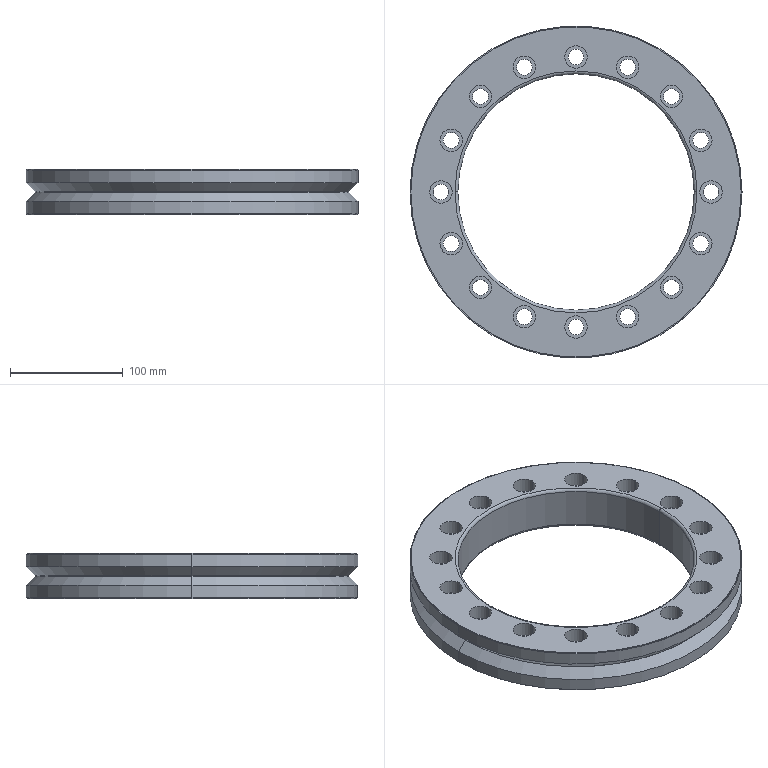Part | SolidWorks | features CirPattern 1, Extrusion 1, Fillet 1, HoleWzd 1, ICE 1, MirrorPattern 1, RefAxis 1, RevCut 1 | 1 solid | 106 faces | box 295 x 295 x 40 mm | volume 1150106 mm3 | cylinder 74 | plane 20 | torus 8 | cone 4 | commonest cylinder face diameters 14 x32 20 x32 293.4 x4 295 x4 210 x2